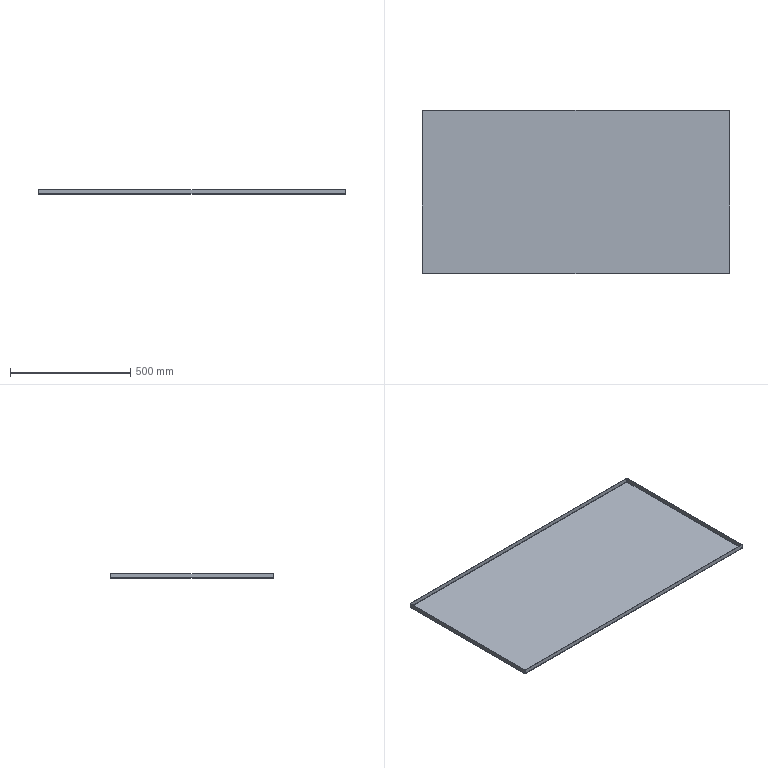Part | STEP file | Part 10 | 1 solid | 38 faces | box 1280 x 680 x 20 mm | volume 1876066 mm3 | plane 22 | spline 8 | cylinder 8 | commonest cylinder face diameters 1 x4 5 x4
STEP:
#1=CARTESIAN_POINT('',(-637.5,-337.5,-2.));
#2=VERTEX_POINT('',#1);
#3=CARTESIAN_POINT('',(-637.5,337.5,-2.));
#4=VERTEX_POINT('',#3);
#5=CARTESIAN_POINT('',(-637.5,-337.5,-2.));
#6=DIRECTION('',(0.,1.,0.));
#7=VECTOR('',#6,1000.);
#8=LINE('',#5,#7);
#9=EDGE_CURVE('',#2,#4,#8,.T.);
#10=ORIENTED_EDGE('',*,*,#9,.T.);
#11=CARTESIAN_POINT('',(637.5,337.5,-2.));
#12=VERTEX_POINT('',#11);
#13=CARTESIAN_POINT('',(-637.5,337.5,-2.));
#14=DIRECTION('',(1.,0.,0.));
#15=VECTOR('',#14,1000.);
#16=LINE('',#13,#15);
#17=EDGE_CURVE('',#4,#12,#16,.T.);
#18=ORIENTED_EDGE('',*,*,#17,.T.);
#19=CARTESIAN_POINT('',(637.5,-337.5,-2.));
#20=VERTEX_POINT('',#19);
#21=CARTESIAN_POINT('',(637.5,337.5,-2.));
#22=DIRECTION('',(0.,-1.,0.));
#23=VECTOR('',#22,1000.);
#24=LINE('',#21,#23);
#25=EDGE_CURVE('',#12,#20,#24,.T.);
#26=ORIENTED_EDGE('',*,*,#25,.T.);
#27=CARTESIAN_POINT('',(637.5,-337.5,-2.));
#28=DIRECTION('',(-1.,0.,0.));
#29=VECTOR('',#28,1000.);
#30=LINE('',#27,#29);
#31=EDGE_CURVE('',#20,#2,#30,.T.);
#32=ORIENTED_EDGE('',*,*,#31,.T.);
#33=EDGE_LOOP('',(#10,#18,#26,#32));
#34=FACE_OUTER_BOUND('',#33,.T.);
#35=CARTESIAN_POINT('',(0.,0.,-2.));
#36=DIRECTION('',(0.,0.,1.));
#37=DIRECTION('',(1.,0.,0.));
#38=AXIS2_PLACEMENT_3D('',#35,#36,#37);
#39=PLANE('',#38);
#40=ADVANCED_FACE('',(#34),#39,.F.);
#41=CARTESIAN_POINT('',(-637.5,337.5,0.));
#42=VERTEX_POINT('',#41);
#43=CARTESIAN_POINT('',(637.5,337.5,0.));
#44=VERTEX_POINT('',#43);
#45=CARTESIAN_POINT('',(-637.5,337.5,0.));
#46=DIRECTION('',(1.,0.,0.));
#47=VECTOR('',#46,1000.);
#48=LINE('',#45,#47);
#49=EDGE_CURVE('',#42,#44,#48,.T.);
#50=ORIENTED_EDGE('',*,*,#49,.F.);
#51=CARTESIAN_POINT('',(-637.5,-337.5,0.));
#52=VERTEX_POINT('',#51);
#53=CARTESIAN_POINT('',(-637.5,-337.5,0.));
#54=DIRECTION('',(0.,1.,0.));
#55=VECTOR('',#54,1000.);
#56=LINE('',#53,#55);
#57=EDGE_CURVE('',#52,#42,#56,.T.);
#58=ORIENTED_EDGE('',*,*,#57,.F.);
#59=CARTESIAN_POINT('',(637.5,-337.5,0.));
#60=VERTEX_POINT('',#59);
#61=CARTESIAN_POINT('',(637.5,-337.5,0.));
#62=DIRECTION('',(-1.,0.,0.));
#63=VECTOR('',#62,1000.);
#64=LINE('',#61,#63);
#65=EDGE_CURVE('',#60,#52,#64,.T.);
#66=ORIENTED_EDGE('',*,*,#65,.F.);
#67=CARTESIAN_POINT('',(637.5,337.5,0.));
#68=DIRECTION('',(0.,-1.,0.));
#69=VECTOR('',#68,1000.);
#70=LINE('',#67,#69);
#71=EDGE_CURVE('',#44,#60,#70,.T.);
#72=ORIENTED_EDGE('',*,*,#71,.F.);
#73=EDGE_LOOP('',(#50,#58,#66,#72));
#74=FACE_OUTER_BOUND('',#73,.T.);
#75=CARTESIAN_POINT('',(0.,0.,0.));
#76=DIRECTION('',(0.,0.,1.));
#77=DIRECTION('',(1.,0.,0.));
#78=AXIS2_PLACEMENT_3D('',#75,#76,#77);
#79=PLANE('',#78);
#80=ADVANCED_FACE('',(#74),#79,.T.);
#81=CARTESIAN_POINT('',(637.293,340.,0.5));
#82=VERTEX_POINT('',#81);
#83=CARTESIAN_POINT('',(637.293,338.,0.5));
#84=VERTEX_POINT('',#83);
#85=CARTESIAN_POINT('',(637.293,338.,0.5));
#86=DIRECTION('',(0.,-1.,0.));
#87=VECTOR('',#86,1000.);
#88=LINE('',#85,#87);
#89=EDGE_CURVE('',#82,#84,#88,.T.);
#90=ORIENTED_EDGE('',*,*,#89,.T.);
#91=CARTESIAN_POINT('',(637.5,337.5,0.));
#92=CARTESIAN_POINT('',(637.465,337.631,0.));
#93=CARTESIAN_POINT('',(637.431,337.761,0.05389));
#94=CARTESIAN_POINT('',(637.362,337.946,0.239));
#95=CARTESIAN_POINT('',(637.327,338.,0.3691));
#96=CARTESIAN_POINT('',(637.293,338.,0.5));
#97=B_SPLINE_CURVE_WITH_KNOTS('',3,(#91,#92,#93,#94,#95,#96),.UNSPECIFIED.,.F.,.F.,(4,2,4),(0.,0.5,1.),.UNSPECIFIED.);
#98=EDGE_CURVE('',#44,#84,#97,.T.);
#99=ORIENTED_EDGE('',*,*,#98,.F.);
#100=CARTESIAN_POINT('',(637.5,337.5,0.));
#101=DIRECTION('',(0.,0.,-1.));
#102=VECTOR('',#101,1000.);
#103=LINE('',#100,#102);
#104=EDGE_CURVE('',#44,#12,#103,.T.);
#105=ORIENTED_EDGE('',*,*,#104,.T.);
#106=CARTESIAN_POINT('',(637.5,337.5,-2.));
#107=CARTESIAN_POINT('',(637.483,337.827,-2.));
#108=CARTESIAN_POINT('',(637.465,338.154,-1.935));
#109=CARTESIAN_POINT('',(637.431,338.759,-1.684));
#110=CARTESIAN_POINT('',(637.414,339.036,-1.499));
#111=CARTESIAN_POINT('',(637.379,339.499,-1.036));
#112=CARTESIAN_POINT('',(637.362,339.684,-0.759));
#113=CARTESIAN_POINT('',(637.327,339.935,-0.1544));
#114=CARTESIAN_POINT('',(637.31,340.,0.1728));
#115=CARTESIAN_POINT('',(637.293,340.,0.5));
#116=B_SPLINE_CURVE_WITH_KNOTS('',3,(#106,#107,#108,#109,#110,#111,#112,#113,#114,#115),.UNSPECIFIED.,.F.,.F.,(4,2,2,2,4),(0.,0.25,0.5,0.75,1.),.UNSPECIFIED.);
#117=EDGE_CURVE('',#12,#82,#116,.T.);
#118=ORIENTED_EDGE('',*,*,#117,.T.);
#119=EDGE_LOOP('',(#90,#99,#105,#118));
#120=FACE_OUTER_BOUND('',#119,.T.);
#121=CARTESIAN_POINT('',(637.5,337.5,-2.02));
#122=CARTESIAN_POINT('',(637.483,337.83,-2.02));
#123=CARTESIAN_POINT('',(637.465,338.16,-1.954));
#124=CARTESIAN_POINT('',(637.431,338.769,-1.702));
#125=CARTESIAN_POINT('',(637.414,339.049,-1.515));
#126=CARTESIAN_POINT('',(637.379,339.515,-1.049));
#127=CARTESIAN_POINT('',(637.362,339.702,-0.7691));
#128=CARTESIAN_POINT('',(637.327,339.954,-0.1596));
#129=CARTESIAN_POINT('',(637.31,340.02,0.1701));
#130=CARTESIAN_POINT('',(637.293,340.02,0.5));
#131=CARTESIAN_POINT('',(637.5,337.5,-2.));
#132=CARTESIAN_POINT('',(637.483,337.827,-2.));
#133=CARTESIAN_POINT('',(637.465,338.154,-1.935));
#134=CARTESIAN_POINT('',(637.431,338.759,-1.684));
#135=CARTESIAN_POINT('',(637.414,339.036,-1.499));
#136=CARTESIAN_POINT('',(637.379,339.499,-1.036));
#137=CARTESIAN_POINT('',(637.362,339.684,-0.759));
#138=CARTESIAN_POINT('',(637.327,339.935,-0.1544));
#139=CARTESIAN_POINT('',(637.31,340.,0.1727));
#140=CARTESIAN_POINT('',(637.293,340.,0.5));
#141=CARTESIAN_POINT('',(637.5,337.5,0.));
#142=CARTESIAN_POINT('',(637.483,337.565,0.));
#143=CARTESIAN_POINT('',(637.465,337.631,0.01301));
#144=CARTESIAN_POINT('',(637.431,337.752,0.06311));
#145=CARTESIAN_POINT('',(637.414,337.807,0.1002));
#146=CARTESIAN_POINT('',(637.379,337.9,0.1927));
#147=CARTESIAN_POINT('',(637.362,337.937,0.2482));
#148=CARTESIAN_POINT('',(637.327,337.987,0.3691));
#149=CARTESIAN_POINT('',(637.31,338.,0.4345));
#150=CARTESIAN_POINT('',(637.293,338.,0.5));
#151=CARTESIAN_POINT('',(637.5,337.5,0.0202));
#152=CARTESIAN_POINT('',(637.483,337.563,0.0202));
#153=CARTESIAN_POINT('',(637.465,337.626,0.03269));
#154=CARTESIAN_POINT('',(637.431,337.742,0.08076));
#155=CARTESIAN_POINT('',(637.414,337.795,0.1163));
#156=CARTESIAN_POINT('',(637.379,337.884,0.2051));
#157=CARTESIAN_POINT('',(637.362,337.919,0.2584));
#158=CARTESIAN_POINT('',(637.327,337.967,0.3744));
#159=CARTESIAN_POINT('',(637.31,337.98,0.4372));
#160=CARTESIAN_POINT('',(637.293,337.98,0.5));
#161=B_SPLINE_SURFACE_WITH_KNOTS('',1,3,((#121,#122,#123,#124,#125,#126,#127,#128,#129,#130),(#131,#132,#133,#134,#135,#136,#137,#138,#139,#140),(#141,#142,#143,#144,#145,#146,#147,#148,#149,#150),(#151,#152,#153,#154,#155,#156,#157,#158,#159,#160)),.UNSPECIFIED.,.F.,.F.,.F.,(2,1,1,2),(4,2,2,2,4),(-0.01,0.,1.,1.01),(0.,0.25,0.5,0.75,1.),.UNSPECIFIED.);
#162=ADVANCED_FACE('',(#120),#161,.F.);
#163=CARTESIAN_POINT('',(-637.293,338.,0.5));
#164=VERTEX_POINT('',#163);
#165=CARTESIAN_POINT('',(-637.293,338.,0.5));
#166=CARTESIAN_POINT('',(-637.327,338.,0.3691));
#167=CARTESIAN_POINT('',(-637.362,337.946,0.239));
#168=CARTESIAN_POINT('',(-637.431,337.761,0.05389));
#169=CARTESIAN_POINT('',(-637.465,337.631,0.));
#170=CARTESIAN_POINT('',(-637.5,337.5,0.));
#171=B_SPLINE_CURVE_WITH_KNOTS('',3,(#165,#166,#167,#168,#169,#170),.UNSPECIFIED.,.F.,.F.,(4,2,4),(0.,0.5,1.),.UNSPECIFIED.);
#172=EDGE_CURVE('',#164,#42,#171,.T.);
#173=ORIENTED_EDGE('',*,*,#172,.F.);
#174=CARTESIAN_POINT('',(-637.293,340.,0.5));
#175=VERTEX_POINT('',#174);
#176=CARTESIAN_POINT('',(-637.293,338.,0.5));
#177=DIRECTION('',(0.,-1.,0.));
#178=VECTOR('',#177,1000.);
#179=LINE('',#176,#178);
#180=EDGE_CURVE('',#175,#164,#179,.T.);
#181=ORIENTED_EDGE('',*,*,#180,.F.);
#182=CARTESIAN_POINT('',(-637.293,340.,0.5));
#183=CARTESIAN_POINT('',(-637.31,340.,0.1728));
#184=CARTESIAN_POINT('',(-637.327,339.935,-0.1544));
#185=CARTESIAN_POINT('',(-637.362,339.684,-0.759));
#186=CARTESIAN_POINT('',(-637.379,339.499,-1.036));
#187=CARTESIAN_POINT('',(-637.414,339.036,-1.499));
#188=CARTESIAN_POINT('',(-637.431,338.759,-1.684));
#189=CARTESIAN_POINT('',(-637.465,338.154,-1.935));
#190=CARTESIAN_POINT('',(-637.483,337.827,-2.));
#191=CARTESIAN_POINT('',(-637.5,337.5,-2.));
#192=B_SPLINE_CURVE_WITH_KNOTS('',3,(#182,#183,#184,#185,#186,#187,#188,#189,#190,#191),.UNSPECIFIED.,.F.,.F.,(4,2,2,2,4),(0.,0.25,0.5,0.75,1.),.UNSPECIFIED.);
#193=EDGE_CURVE('',#175,#4,#192,.T.);
#194=ORIENTED_EDGE('',*,*,#193,.T.);
#195=CARTESIAN_POINT('',(-637.5,337.5,0.));
#196=DIRECTION('',(0.,0.,-1.));
#197=VECTOR('',#196,1000.);
#198=LINE('',#195,#197);
#199=EDGE_CURVE('',#42,#4,#198,.T.);
#200=ORIENTED_EDGE('',*,*,#199,.F.);
#201=EDGE_LOOP('',(#173,#181,#194,#200));
#202=FACE_OUTER_BOUND('',#201,.T.);
#203=CARTESIAN_POINT('',(-637.293,340.02,0.5));
#204=CARTESIAN_POINT('',(-637.31,340.02,0.1701));
#205=CARTESIAN_POINT('',(-637.327,339.954,-0.1596));
#206=CARTESIAN_POINT('',(-637.362,339.702,-0.7691));
#207=CARTESIAN_POINT('',(-637.379,339.515,-1.049));
#208=CARTESIAN_POINT('',(-637.414,339.049,-1.515));
#209=CARTESIAN_POINT('',(-637.431,338.769,-1.702));
#210=CARTESIAN_POINT('',(-637.465,338.16,-1.954));
#211=CARTESIAN_POINT('',(-637.483,337.83,-2.02));
#212=CARTESIAN_POINT('',(-637.5,337.5,-2.02));
#213=CARTESIAN_POINT('',(-637.293,340.,0.5));
#214=CARTESIAN_POINT('',(-637.31,340.,0.1727));
#215=CARTESIAN_POINT('',(-637.327,339.935,-0.1544));
#216=CARTESIAN_POINT('',(-637.362,339.684,-0.759));
#217=CARTESIAN_POINT('',(-637.379,339.499,-1.036));
#218=CARTESIAN_POINT('',(-637.414,339.036,-1.499));
#219=CARTESIAN_POINT('',(-637.431,338.759,-1.684));
#220=CARTESIAN_POINT('',(-637.465,338.154,-1.935));
#221=CARTESIAN_POINT('',(-637.483,337.827,-2.));
#222=CARTESIAN_POINT('',(-637.5,337.5,-2.));
#223=CARTESIAN_POINT('',(-637.293,338.,0.5));
#224=CARTESIAN_POINT('',(-637.31,338.,0.4345));
#225=CARTESIAN_POINT('',(-637.327,337.987,0.3691));
#226=CARTESIAN_POINT('',(-637.362,337.937,0.2482));
#227=CARTESIAN_POINT('',(-637.379,337.9,0.1927));
#228=CARTESIAN_POINT('',(-637.414,337.807,0.1002));
#229=CARTESIAN_POINT('',(-637.431,337.752,0.06311));
#230=CARTESIAN_POINT('',(-637.465,337.631,0.01301));
#231=CARTESIAN_POINT('',(-637.483,337.565,0.));
#232=CARTESIAN_POINT('',(-637.5,337.5,0.));
#233=CARTESIAN_POINT('',(-637.293,337.98,0.5));
#234=CARTESIAN_POINT('',(-637.31,337.98,0.4372));
#235=CARTESIAN_POINT('',(-637.327,337.967,0.3744));
#236=CARTESIAN_POINT('',(-637.362,337.919,0.2584));
#237=CARTESIAN_POINT('',(-637.379,337.884,0.2051));
#238=CARTESIAN_POINT('',(-637.414,337.795,0.1163));
#239=CARTESIAN_POINT('',(-637.431,337.742,0.08076));
#240=CARTESIAN_POINT('',(-637.465,337.626,0.03269));
#241=CARTESIAN_POINT('',(-637.483,337.563,0.0202));
#242=CARTESIAN_POINT('',(-637.5,337.5,0.0202));
#243=B_SPLINE_SURFACE_WITH_KNOTS('',1,3,((#203,#204,#205,#206,#207,#208,#209,#210,#211,#212),(#213,#214,#215,#216,#217,#218,#219,#220,#221,#222),(#223,#224,#225,#226,#227,#228,#229,#230,#231,#232),(#233,#234,#235,#236,#237,#238,#239,#240,#241,#242)),.UNSPECIFIED.,.F.,.F.,.F.,(2,1,1,2),(4,2,2,2,4),(-0.01,0.,1.,1.01),(0.,0.25,0.5,0.75,1.),.UNSPECIFIED.);
#244=ADVANCED_FACE('',(#202),#243,.F.);
#245=ORIENTED_EDGE('',*,*,#17,.F.);
#246=ORIENTED_EDGE('',*,*,#193,.F.);
#247=CARTESIAN_POINT('',(0.,340.,0.5));
#248=DIRECTION('',(-1.,0.,0.));
#249=VECTOR('',#248,1000.);
#250=LINE('',#247,#249);
#251=EDGE_CURVE('',#82,#175,#250,.T.);
#252=ORIENTED_EDGE('',*,*,#251,.F.);
#253=ORIENTED_EDGE('',*,*,#117,.F.);
#254=EDGE_LOOP('',(#245,#246,#252,#253));
#255=FACE_OUTER_BOUND('',#254,.T.);
#256=CARTESIAN_POINT('',(-637.5,337.5,0.5));
#257=DIRECTION('',(-1.,0.,0.));
#258=DIRECTION('',(0.,1.,0.));
#259=AXIS2_PLACEMENT_3D('',#256,#257,#258);
#260=CYLINDRICAL_SURFACE('',#259,2.5);
#261=ADVANCED_FACE('',(#255),#260,.T.);
#262=ORIENTED_EDGE('',*,*,#49,.T.);
#263=ORIENTED_EDGE('',*,*,#98,.T.);
#264=CARTESIAN_POINT('',(640.,338.,0.5));
#265=DIRECTION('',(-1.,0.,0.));
#266=VECTOR('',#265,1000.);
#267=LINE('',#264,#266);
#268=EDGE_CURVE('',#84,#164,#267,.T.);
#269=ORIENTED_EDGE('',*,*,#268,.T.);
#270=ORIENTED_EDGE('',*,*,#172,.T.);
#271=EDGE_LOOP('',(#262,#263,#269,#270));
#272=FACE_OUTER_BOUND('',#271,.T.);
#273=CARTESIAN_POINT('',(-637.5,337.5,0.5));
#274=DIRECTION('',(-1.,0.,0.));
#275=DIRECTION('',(0.,1.,0.));
#276=AXIS2_PLACEMENT_3D('',#273,#274,#275);
#277=CYLINDRICAL_SURFACE('',#276,0.5);
#278=ADVANCED_FACE('',(#272),#277,.F.);
#279=CARTESIAN_POINT('',(637.293,338.,18.));
#280=VERTEX_POINT('',#279);
#281=CARTESIAN_POINT('',(637.293,340.,18.));
#282=VERTEX_POINT('',#281);
#283=CARTESIAN_POINT('',(637.293,340.,18.));
#284=DIRECTION('',(0.,1.,0.));
#285=VECTOR('',#284,1000.);
#286=LINE('',#283,#285);
#287=EDGE_CURVE('',#280,#282,#286,.T.);
#288=ORIENTED_EDGE('',*,*,#287,.F.);
#289=CARTESIAN_POINT('',(637.293,338.,0.));
#290=DIRECTION('',(0.,0.,1.));
#291=VECTOR('',#290,1000.);
#292=LINE('',#289,#291);
#293=EDGE_CURVE('',#84,#280,#292,.T.);
#294=ORIENTED_EDGE('',*,*,#293,.F.);
#295=ORIENTED_EDGE('',*,*,#89,.F.);
#296=CARTESIAN_POINT('',(637.293,340.,0.));
#297=DIRECTION('',(0.,0.,-1.));
#298=VECTOR('',#297,1000.);
#299=LINE('',#296,#298);
#300=EDGE_CURVE('',#282,#82,#299,.T.);
#301=ORIENTED_EDGE('',*,*,#300,.F.);
#302=EDGE_LOOP('',(#288,#294,#295,#301));
#303=FACE_OUTER_BOUND('',#302,.T.);
#304=CARTESIAN_POINT('',(637.293,338.,0.));
#305=DIRECTION('',(1.,0.,0.));
#306=DIRECTION('',(0.,0.,-1.));
#307=AXIS2_PLACEMENT_3D('',#304,#305,#306);
#308=PLANE('',#307);
#309=ADVANCED_FACE('',(#303),#308,.T.);
#310=CARTESIAN_POINT('',(-637.293,340.,18.));
#311=VERTEX_POINT('',#310);
#312=CARTESIAN_POINT('',(-637.293,340.,0.));
#313=DIRECTION('',(0.,0.,-1.));
#314=VECTOR('',#313,1000.);
#315=LINE('',#312,#314);
#316=EDGE_CURVE('',#311,#175,#315,.T.);
#317=ORIENTED_EDGE('',*,*,#316,.F.);
#318=CARTESIAN_POINT('',(-640.,340.,18.));
#319=DIRECTION('',(-1.,0.,0.));
#320=VECTOR('',#319,1000.);
#321=LINE('',#318,#320);
#322=EDGE_CURVE('',#282,#311,#321,.T.);
#323=ORIENTED_EDGE('',*,*,#322,.F.);
#324=ORIENTED_EDGE('',*,*,#300,.T.);
#325=ORIENTED_EDGE('',*,*,#251,.T.);
#326=EDGE_LOOP('',(#317,#323,#324,#325));
#327=FACE_OUTER_BOUND('',#326,.T.);
#328=CARTESIAN_POINT('',(0.,340.,0.));
#329=DIRECTION('',(0.,1.,0.));
#330=DIRECTION('',(0.,0.,1.));
#331=AXIS2_PLACEMENT_3D('',#328,#329,#330);
#332=PLANE('',#331);
#333=ADVANCED_FACE('',(#327),#332,.T.);
#334=CARTESIAN_POINT('',(-637.293,338.,18.));
#335=VERTEX_POINT('',#334);
#336=CARTESIAN_POINT('',(0.,338.,18.));
#337=DIRECTION('',(-1.,0.,0.));
#338=VECTOR('',#337,1000.);
#339=LINE('',#336,#338);
#340=EDGE_CURVE('',#280,#335,#339,.T.);
#341=ORIENTED_EDGE('',*,*,#340,.T.);
#342=CARTESIAN_POINT('',(-637.293,338.,0.));
#343=DIRECTION('',(0.,0.,1.));
#344=VECTOR('',#343,1000.);
#345=LINE('',#342,#344);
#346=EDGE_CURVE('',#164,#335,#345,.T.);
#347=ORIENTED_EDGE('',*,*,#346,.F.);
#348=ORIENTED_EDGE('',*,*,#268,.F.);
#349=ORIENTED_EDGE('',*,*,#293,.T.);
#350=EDGE_LOOP('',(#341,#347,#348,#349));
#351=FACE_OUTER_BOUND('',#350,.T.);
#352=CARTESIAN_POINT('',(0.,338.,0.));
#353=DIRECTION('',(0.,1.,0.));
#354=DIRECTION('',(0.,0.,1.));
#355=AXIS2_PLACEMENT_3D('',#352,#353,#354);
#356=PLANE('',#355);
#357=ADVANCED_FACE('',(#351),#356,.F.);
#358=CARTESIAN_POINT('',(-637.293,338.,18.));
#359=DIRECTION('',(0.,1.,0.));
#360=VECTOR('',#359,1000.);
#361=LINE('',#358,#360);
#362=EDGE_CURVE('',#335,#311,#361,.T.);
#363=ORIENTED_EDGE('',*,*,#362,.F.);
#364=ORIENTED_EDGE('',*,*,#340,.F.);
#365=ORIENTED_EDGE('',*,*,#287,.T.);
#366=ORIENTED_EDGE('',*,*,#322,.T.);
#367=EDGE_LOOP('',(#363,#364,#365,#366));
#368=FACE_OUTER_BOUND('',#367,.T.);
#369=CARTESIAN_POINT('',(-640.,340.,18.));
#370=DIRECTION('',(0.,0.,1.));
#371=DIRECTION('',(0.,-1.,0.));
#372=AXIS2_PLACEMENT_3D('',#369,#370,#371);
#373=PLANE('',#372);
#374=ADVANCED_FACE('',(#368),#373,.T.);
#375=ORIENTED_EDGE('',*,*,#346,.T.);
#376=ORIENTED_EDGE('',*,*,#362,.T.);
#377=ORIENTED_EDGE('',*,*,#316,.T.);
#378=ORIENTED_EDGE('',*,*,#180,.T.);
#379=EDGE_LOOP('',(#375,#376,#377,#378));
#380=FACE_OUTER_BOUND('',#379,.T.);
#381=CARTESIAN_POINT('',(-637.293,338.,0.));
#382=DIRECTION('',(1.,0.,0.));
#383=DIRECTION('',(0.,0.,-1.));
#384=AXIS2_PLACEMENT_3D('',#381,#382,#383);
#385=PLANE('',#384);
#386=ADVANCED_FACE('',(#380),#385,.F.);
#387=CARTESIAN_POINT('',(640.,-337.293,0.5));
#388=VERTEX_POINT('',#387);
#389=CARTESIAN_POINT('',(638.,-337.293,0.5));
#390=VERTEX_POINT('',#389);
#391=CARTESIAN_POINT('',(638.,-337.293,0.5));
#392=DIRECTION('',(-1.,0.,0.));
#393=VECTOR('',#392,1000.);
#394=LINE('',#391,#393);
#395=EDGE_CURVE('',#388,#390,#394,.T.);
#396=ORIENTED_EDGE('',*,*,#395,.T.);
#397=CARTESIAN_POINT('',(637.5,-337.5,0.));
#398=CARTESIAN_POINT('',(637.631,-337.465,0.));
#399=CARTESIAN_POINT('',(637.761,-337.431,0.05389));
#400=CARTESIAN_POINT('',(637.946,-337.362,0.239));
#401=CARTESIAN_POINT('',(638.,-337.327,0.3691));
#402=CARTESIAN_POINT('',(638.,-337.293,0.5));
#403=B_SPLINE_CURVE_WITH_KNOTS('',3,(#397,#398,#399,#400,#401,#402),.UNSPECIFIED.,.F.,.F.,(4,2,4),(0.,0.5,1.),.UNSPECIFIED.);
#404=EDGE_CURVE('',#60,#390,#403,.T.);
#405=ORIENTED_EDGE('',*,*,#404,.F.);
#406=CARTESIAN_POINT('',(637.5,-337.5,0.));
#407=DIRECTION('',(0.,0.,-1.));
#408=VECTOR('',#407,1000.);
#409=LINE('',#406,#408);
#410=EDGE_CURVE('',#60,#20,#409,.T.);
#411=ORIENTED_EDGE('',*,*,#410,.T.);
#412=CARTESIAN_POINT('',(637.5,-337.5,-2.));
#413=CARTESIAN_POINT('',(637.827,-337.483,-2.));
#414=CARTESIAN_POINT('',(638.154,-337.465,-1.935));
#415=CARTESIAN_POINT('',(638.759,-337.431,-1.684));
#416=CARTESIAN_POINT('',(639.036,-337.414,-1.499));
#417=CARTESIAN_POINT('',(639.499,-337.379,-1.036));
#418=CARTESIAN_POINT('',(639.684,-337.362,-0.759));
#419=CARTESIAN_POINT('',(639.935,-337.327,-0.1544));
#420=CARTESIAN_POINT('',(640.,-337.31,0.1728));
#421=CARTESIAN_POINT('',(640.,-337.293,0.5));
#422=B_SPLINE_CURVE_WITH_KNOTS('',3,(#412,#413,#414,#415,#416,#417,#418,#419,#420,#421),.UNSPECIFIED.,.F.,.F.,(4,2,2,2,4),(0.,0.25,0.5,0.75,1.),.UNSPECIFIED.);
#423=EDGE_CURVE('',#20,#388,#422,.T.);
#424=ORIENTED_EDGE('',*,*,#423,.T.);
#425=EDGE_LOOP('',(#396,#405,#411,#424));
#426=FACE_OUTER_BOUND('',#425,.T.);
#427=CARTESIAN_POINT('',(637.5,-337.5,-2.02));
#428=CARTESIAN_POINT('',(637.83,-337.483,-2.02));
#429=CARTESIAN_POINT('',(638.16,-337.465,-1.954));
#430=CARTESIAN_POINT('',(638.769,-337.431,-1.702));
#431=CARTESIAN_POINT('',(639.049,-337.414,-1.515));
#432=CARTESIAN_POINT('',(639.515,-337.379,-1.049));
#433=CARTESIAN_POINT('',(639.702,-337.362,-0.7691));
#434=CARTESIAN_POINT('',(639.954,-337.327,-0.1596));
#435=CARTESIAN_POINT('',(640.02,-337.31,0.1701));
#436=CARTESIAN_POINT('',(640.02,-337.293,0.5));
#437=CARTESIAN_POINT('',(637.5,-337.5,-2.));
#438=CARTESIAN_POINT('',(637.827,-337.483,-2.));
#439=CARTESIAN_POINT('',(638.154,-337.465,-1.935));
#440=CARTESIAN_POINT('',(638.759,-337.431,-1.684));
#441=CARTESIAN_POINT('',(639.036,-337.414,-1.499));
#442=CARTESIAN_POINT('',(639.499,-337.379,-1.036));
#443=CARTESIAN_POINT('',(639.684,-337.362,-0.759));
#444=CARTESIAN_POINT('',(639.935,-337.327,-0.1544));
#445=CARTESIAN_POINT('',(640.,-337.31,0.1727));
#446=CARTESIAN_POINT('',(640.,-337.293,0.5));
#447=CARTESIAN_POINT('',(637.5,-337.5,0.));
#448=CARTESIAN_POINT('',(637.565,-337.483,0.));
#449=CARTESIAN_POINT('',(637.631,-337.465,0.01301));
#450=CARTESIAN_POINT('',(637.752,-337.431,0.06311));
#451=CARTESIAN_POINT('',(637.807,-337.414,0.1002));
#452=CARTESIAN_POINT('',(637.9,-337.379,0.1927));
#453=CARTESIAN_POINT('',(637.937,-337.362,0.2482));
#454=CARTESIAN_POINT('',(637.987,-337.327,0.3691));
#455=CARTESIAN_POINT('',(638.,-337.31,0.4345));
#456=CARTESIAN_POINT('',(638.,-337.293,0.5));
#457=CARTESIAN_POINT('',(637.5,-337.5,0.0202));
#458=CARTESIAN_POINT('',(637.563,-337.483,0.0202));
#459=CARTESIAN_POINT('',(637.626,-337.465,0.03269));
#460=CARTESIAN_POINT('',(637.742,-337.431,0.08076));
#461=CARTESIAN_POINT('',(637.795,-337.414,0.1163));
#462=CARTESIAN_POINT('',(637.884,-337.379,0.2051));
#463=CARTESIAN_POINT('',(637.919,-337.362,0.2584));
#464=CARTESIAN_POINT('',(637.967,-337.327,0.3744));
#465=CARTESIAN_POINT('',(637.98,-337.31,0.4372));
#466=CARTESIAN_POINT('',(637.98,-337.293,0.5));
#467=B_SPLINE_SURFACE_WITH_KNOTS('',1,3,((#427,#428,#429,#430,#431,#432,#433,#434,#435,#436),(#437,#438,#439,#440,#441,#442,#443,#444,#445,#446),(#447,#448,#449,#450,#451,#452,#453,#454,#455,#456),(#457,#458,#459,#460,#461,#462,#463,#464,#465,#466)),.UNSPECIFIED.,.F.,.F.,.F.,(2,1,1,2),(4,2,2,2,4),(-0.01,0.,1.,1.01),(0.,0.25,0.5,0.75,1.),.UNSPECIFIED.);
#468=ADVANCED_FACE('',(#426),#467,.F.);
#469=CARTESIAN_POINT('',(638.,337.293,0.5));
#470=VERTEX_POINT('',#469);
#471=CARTESIAN_POINT('',(638.,337.293,0.5));
#472=CARTESIAN_POINT('',(638.,337.327,0.3691));
#473=CARTESIAN_POINT('',(637.946,337.362,0.239));
#474=CARTESIAN_POINT('',(637.761,337.431,0.05389));
#475=CARTESIAN_POINT('',(637.631,337.465,0.));
#476=CARTESIAN_POINT('',(637.5,337.5,0.));
#477=B_SPLINE_CURVE_WITH_KNOTS('',3,(#471,#472,#473,#474,#475,#476),.UNSPECIFIED.,.F.,.F.,(4,2,4),(0.,0.5,1.),.UNSPECIFIED.);
#478=EDGE_CURVE('',#470,#44,#477,.T.);
#479=ORIENTED_EDGE('',*,*,#478,.F.);
#480=CARTESIAN_POINT('',(640.,337.293,0.5));
#481=VERTEX_POINT('',#480);
#482=CARTESIAN_POINT('',(638.,337.293,0.5));
#483=DIRECTION('',(-1.,0.,0.));
#484=VECTOR('',#483,1000.);
#485=LINE('',#482,#484);
#486=EDGE_CURVE('',#481,#470,#485,.T.);
#487=ORIENTED_EDGE('',*,*,#486,.F.);
#488=CARTESIAN_POINT('',(640.,337.293,0.5));
#489=CARTESIAN_POINT('',(640.,337.31,0.1728));
#490=CARTESIAN_POINT('',(639.935,337.327,-0.1544));
#491=CARTESIAN_POINT('',(639.684,337.362,-0.759));
#492=CARTESIAN_POINT('',(639.499,337.379,-1.036));
#493=CARTESIAN_POINT('',(639.036,337.414,-1.499));
#494=CARTESIAN_POINT('',(638.759,337.431,-1.684));
#495=CARTESIAN_POINT('',(638.154,337.465,-1.935));
#496=CARTESIAN_POINT('',(637.827,337.483,-2.));
#497=CARTESIAN_POINT('',(637.5,337.5,-2.));
#498=B_SPLINE_CURVE_WITH_KNOTS('',3,(#488,#489,#490,#491,#492,#493,#494,#495,#496,#497),.UNSPECIFIED.,.F.,.F.,(4,2,2,2,4),(0.,0.25,0.5,0.75,1.),.UNSPECIFIED.);
#499=EDGE_CURVE('',#481,#12,#498,.T.);
#500=ORIENTED_EDGE('',*,*,#499,.T.);
#501=ORIENTED_EDGE('',*,*,#104,.F.);
#502=EDGE_LOOP('',(#479,#487,#500,#501));
#503=FACE_OUTER_BOUND('',#502,.T.);
#504=CARTESIAN_POINT('',(640.02,337.293,0.5));
#505=CARTESIAN_POINT('',(640.02,337.31,0.1701));
#506=CARTESIAN_POINT('',(639.954,337.327,-0.1596));
#507=CARTESIAN_POINT('',(639.702,337.362,-0.7691));
#508=CARTESIAN_POINT('',(639.515,337.379,-1.049));
#509=CARTESIAN_POINT('',(639.049,337.414,-1.515));
#510=CARTESIAN_POINT('',(638.769,337.431,-1.702));
#511=CARTESIAN_POINT('',(638.16,337.465,-1.954));
#512=CARTESIAN_POINT('',(637.83,337.483,-2.02));
#513=CARTESIAN_POINT('',(637.5,337.5,-2.02));
#514=CARTESIAN_POINT('',(640.,337.293,0.5));
#515=CARTESIAN_POINT('',(640.,337.31,0.1727));
#516=CARTESIAN_POINT('',(639.935,337.327,-0.1544));
#517=CARTESIAN_POINT('',(639.684,337.362,-0.759));
#518=CARTESIAN_POINT('',(639.499,337.379,-1.036));
#519=CARTESIAN_POINT('',(639.036,337.414,-1.499));
#520=CARTESIAN_POINT('',(638.759,337.431,-1.684));
#521=CARTESIAN_POINT('',(638.154,337.465,-1.935));
#522=CARTESIAN_POINT('',(637.827,337.483,-2.));
#523=CARTESIAN_POINT('',(637.5,337.5,-2.));
#524=CARTESIAN_POINT('',(638.,337.293,0.5));
#525=CARTESIAN_POINT('',(638.,337.31,0.4345));
#526=CARTESIAN_POINT('',(637.987,337.327,0.3691));
#527=CARTESIAN_POINT('',(637.937,337.362,0.2482));
#528=CARTESIAN_POINT('',(637.9,337.379,0.1927));
#529=CARTESIAN_POINT('',(637.807,337.414,0.1002));
#530=CARTESIAN_POINT('',(637.752,337.431,0.06311));
#531=CARTESIAN_POINT('',(637.631,337.465,0.01301));
#532=CARTESIAN_POINT('',(637.565,337.483,0.));
#533=CARTESIAN_POINT('',(637.5,337.5,0.));
#534=CARTESIAN_POINT('',(637.98,337.293,0.5));
#535=CARTESIAN_POINT('',(637.98,337.31,0.4372));
#536=CARTESIAN_POINT('',(637.967,337.327,0.3744));
#537=CARTESIAN_POINT('',(637.919,337.362,0.2584));
#538=CARTESIAN_POINT('',(637.884,337.379,0.2051));
#539=CARTESIAN_POINT('',(637.795,337.414,0.1163));
#540=CARTESIAN_POINT('',(637.742,337.431,0.08076));
#541=CARTESIAN_POINT('',(637.626,337.465,0.03269));
#542=CARTESIAN_POINT('',(637.563,337.483,0.0202));
#543=CARTESIAN_POINT('',(637.5,337.5,0.0202));
#544=B_SPLINE_SURFACE_WITH_KNOTS('',1,3,((#504,#505,#506,#507,#508,#509,#510,#511,#512,#513),(#514,#515,#516,#517,#518,#519,#520,#521,#522,#523),(#524,#525,#526,#527,#528,#529,#530,#531,#532,#533),(#534,#535,#536,#537,#538,#539,#540,#541,#542,#543)),.UNSPECIFIED.,.F.,.F.,.F.,(2,1,1,2),(4,2,2,2,4),(-0.01,0.,1.,1.01),(0.,0.25,0.5,0.75,1.),.UNSPECIFIED.);
#545=ADVANCED_FACE('',(#503),#544,.F.);
#546=ORIENTED_EDGE('',*,*,#25,.F.);
#547=ORIENTED_EDGE('',*,*,#499,.F.);
#548=CARTESIAN_POINT('',(640.,-340.,0.5));
#549=DIRECTION('',(0.,-1.,0.));
#550=VECTOR('',#549,1000.);
#551=LINE('',#548,#550);
#552=EDGE_CURVE('',#481,#388,#551,.T.);
#553=ORIENTED_EDGE('',*,*,#552,.T.);
#554=ORIENTED_EDGE('',*,*,#423,.F.);
#555=EDGE_LOOP('',(#546,#547,#553,#554));
#556=FACE_OUTER_BOUND('',#555,.T.);
#557=CARTESIAN_POINT('',(637.5,337.5,0.5));
#558=DIRECTION('',(0.,1.,0.));
#559=DIRECTION('',(1.,0.,0.));
#560=AXIS2_PLACEMENT_3D('',#557,#558,#559);
#561=CYLINDRICAL_SURFACE('',#560,2.5);
#562=ADVANCED_FACE('',(#556),#561,.T.);
#563=ORIENTED_EDGE('',*,*,#71,.T.);
#564=ORIENTED_EDGE('',*,*,#404,.T.);
#565=CARTESIAN_POINT('',(638.,-340.,0.5));
#566=DIRECTION('',(0.,1.,0.));
#567=VECTOR('',#566,1000.);
#568=LINE('',#565,#567);
#569=EDGE_CURVE('',#390,#470,#568,.T.);
#570=ORIENTED_EDGE('',*,*,#569,.T.);
#571=ORIENTED_EDGE('',*,*,#478,.T.);
#572=EDGE_LOOP('',(#563,#564,#570,#571));
#573=FACE_OUTER_BOUND('',#572,.T.);
#574=CARTESIAN_POINT('',(637.5,337.5,0.5));
#575=DIRECTION('',(0.,1.,0.));
#576=DIRECTION('',(1.,0.,0.));
#577=AXIS2_PLACEMENT_3D('',#574,#575,#576);
#578=CYLINDRICAL_SURFACE('',#577,0.5);
#579=ADVANCED_FACE('',(#573),#578,.F.);
#580=CARTESIAN_POINT('',(638.,-337.293,18.));
#581=VERTEX_POINT('',#580);
#582=CARTESIAN_POINT('',(640.,-337.293,18.));
#583=VERTEX_POINT('',#582);
#584=CARTESIAN_POINT('',(640.,-337.293,18.));
#585=DIRECTION('',(1.,0.,0.));
#586=VECTOR('',#585,1000.);
#587=LINE('',#584,#586);
#588=EDGE_CURVE('',#581,#583,#587,.T.);
#589=ORIENTED_EDGE('',*,*,#588,.F.);
#590=CARTESIAN_POINT('',(638.,-337.293,0.));
#591=DIRECTION('',(0.,0.,1.));
#592=VECTOR('',#591,1000.);
#593=LINE('',#590,#592);
#594=EDGE_CURVE('',#390,#581,#593,.T.);
#595=ORIENTED_EDGE('',*,*,#594,.F.);
#596=ORIENTED_EDGE('',*,*,#395,.F.);
#597=CARTESIAN_POINT('',(640.,-337.293,0.));
#598=DIRECTION('',(0.,0.,1.));
#599=VECTOR('',#598,1000.);
#600=LINE('',#597,#599);
#601=EDGE_CURVE('',#388,#583,#600,.T.);
#602=ORIENTED_EDGE('',*,*,#601,.T.);
#603=EDGE_LOOP('',(#589,#595,#596,#602));
#604=FACE_OUTER_BOUND('',#603,.T.);
#605=CARTESIAN_POINT('',(638.,-337.293,0.));
#606=DIRECTION('',(0.,-1.,0.));
#607=DIRECTION('',(0.,0.,-1.));
#608=AXIS2_PLACEMENT_3D('',#605,#606,#607);
#609=PLANE('',#608);
#610=ADVANCED_FACE('',(#604),#609,.T.);
#611=ORIENTED_EDGE('',*,*,#552,.F.);
#612=CARTESIAN_POINT('',(640.,337.293,18.));
#613=VERTEX_POINT('',#612);
#614=CARTESIAN_POINT('',(640.,337.293,0.));
#615=DIRECTION('',(0.,0.,1.));
#616=VECTOR('',#615,1000.);
#617=LINE('',#614,#616);
#618=EDGE_CURVE('',#481,#613,#617,.T.);
#619=ORIENTED_EDGE('',*,*,#618,.T.);
#620=CARTESIAN_POINT('',(640.,-340.,18.));
#621=DIRECTION('',(0.,1.,0.));
#622=VECTOR('',#621,1000.);
#623=LINE('',#620,#622);
#624=EDGE_CURVE('',#583,#613,#623,.T.);
#625=ORIENTED_EDGE('',*,*,#624,.F.);
#626=ORIENTED_EDGE('',*,*,#601,.F.);
#627=EDGE_LOOP('',(#611,#619,#625,#626));
#628=FACE_OUTER_BOUND('',#627,.T.);
#629=CARTESIAN_POINT('',(640.,0.,0.));
#630=DIRECTION('',(-1.,0.,0.));
#631=DIRECTION('',(0.,0.,1.));
#632=AXIS2_PLACEMENT_3D('',#629,#630,#631);
#633=PLANE('',#632);
#634=ADVANCED_FACE('',(#628),#633,.F.);
#635=CARTESIAN_POINT('',(638.,337.293,18.));
#636=VERTEX_POINT('',#635);
#637=CARTESIAN_POINT('',(638.,337.293,0.));
#638=DIRECTION('',(0.,0.,1.));
#639=VECTOR('',#638,1000.);
#640=LINE('',#637,#639);
#641=EDGE_CURVE('',#470,#636,#640,.T.);
#642=ORIENTED_EDGE('',*,*,#641,.F.);
#643=ORIENTED_EDGE('',*,*,#569,.F.);
#644=ORIENTED_EDGE('',*,*,#594,.T.);
#645=CARTESIAN_POINT('',(638.,0.,18.));
#646=DIRECTION('',(0.,1.,0.));
#647=VECTOR('',#646,1000.);
#648=LINE('',#645,#647);
#649=EDGE_CURVE('',#581,#636,#648,.T.);
#650=ORIENTED_EDGE('',*,*,#649,.T.);
#651=EDGE_LOOP('',(#642,#643,#644,#650));
#652=FACE_OUTER_BOUND('',#651,.T.);
#653=CARTESIAN_POINT('',(638.,0.,0.));
#654=DIRECTION('',(-1.,0.,0.));
#655=DIRECTION('',(0.,0.,1.));
#656=AXIS2_PLACEMENT_3D('',#653,#654,#655);
#657=PLANE('',#656);
#658=ADVANCED_FACE('',(#652),#657,.T.);
#659=CARTESIAN_POINT('',(638.,337.293,18.));
#660=DIRECTION('',(1.,0.,0.));
#661=VECTOR('',#660,1000.);
#662=LINE('',#659,#661);
#663=EDGE_CURVE('',#636,#613,#662,.T.);
#664=ORIENTED_EDGE('',*,*,#663,.F.);
#665=ORIENTED_EDGE('',*,*,#649,.F.);
#666=ORIENTED_EDGE('',*,*,#588,.T.);
#667=ORIENTED_EDGE('',*,*,#624,.T.);
#668=EDGE_LOOP('',(#664,#665,#666,#667));
#669=FACE_OUTER_BOUND('',#668,.T.);
#670=CARTESIAN_POINT('',(640.,-340.,18.));
#671=DIRECTION('',(0.,0.,1.));
#672=DIRECTION('',(1.,0.,0.));
#673=AXIS2_PLACEMENT_3D('',#670,#671,#672);
#674=PLANE('',#673);
#675=ADVANCED_FACE('',(#669),#674,.T.);
#676=ORIENTED_EDGE('',*,*,#641,.T.);
#677=ORIENTED_EDGE('',*,*,#663,.T.);
#678=ORIENTED_EDGE('',*,*,#618,.F.);
#679=ORIENTED_EDGE('',*,*,#486,.T.);
#680=EDGE_LOOP('',(#676,#677,#678,#679));
#681=FACE_OUTER_BOUND('',#680,.T.);
#682=CARTESIAN_POINT('',(638.,337.293,0.));
#683=DIRECTION('',(0.,-1.,0.));
#684=DIRECTION('',(0.,0.,-1.));
#685=AXIS2_PLACEMENT_3D('',#682,#683,#684);
#686=PLANE('',#685);
#687=ADVANCED_FACE('',(#681),#686,.F.);
#688=CARTESIAN_POINT('',(-637.293,-340.,0.5));
#689=VERTEX_POINT('',#688);
#690=CARTESIAN_POINT('',(-637.293,-338.,0.5));
#691=VERTEX_POINT('',#690);
#692=CARTESIAN_POINT('',(-637.293,-338.,0.5));
#693=DIRECTION('',(0.,1.,0.));
#694=VECTOR('',#693,1000.);
#695=LINE('',#692,#694);
#696=EDGE_CURVE('',#689,#691,#695,.T.);
#697=ORIENTED_EDGE('',*,*,#696,.T.);
#698=CARTESIAN_POINT('',(-637.5,-337.5,0.));
#699=CARTESIAN_POINT('',(-637.465,-337.631,0.));
#700=CARTESIAN_POINT('',(-637.431,-337.761,0.05389));
#701=CARTESIAN_POINT('',(-637.362,-337.946,0.239));
#702=CARTESIAN_POINT('',(-637.327,-338.,0.3691));
#703=CARTESIAN_POINT('',(-637.293,-338.,0.5));
#704=B_SPLINE_CURVE_WITH_KNOTS('',3,(#698,#699,#700,#701,#702,#703),.UNSPECIFIED.,.F.,.F.,(4,2,4),(0.,0.5,1.),.UNSPECIFIED.);
#705=EDGE_CURVE('',#52,#691,#704,.T.);
#706=ORIENTED_EDGE('',*,*,#705,.F.);
#707=CARTESIAN_POINT('',(-637.5,-337.5,0.));
#708=DIRECTION('',(0.,0.,-1.));
#709=VECTOR('',#708,1000.);
#710=LINE('',#707,#709);
#711=EDGE_CURVE('',#52,#2,#710,.T.);
#712=ORIENTED_EDGE('',*,*,#711,.T.);
#713=CARTESIAN_POINT('',(-637.5,-337.5,-2.));
#714=CARTESIAN_POINT('',(-637.483,-337.827,-2.));
#715=CARTESIAN_POINT('',(-637.465,-338.154,-1.935));
#716=CARTESIAN_POINT('',(-637.431,-338.759,-1.684));
#717=CARTESIAN_POINT('',(-637.414,-339.036,-1.499));
#718=CARTESIAN_POINT('',(-637.379,-339.499,-1.036));
#719=CARTESIAN_POINT('',(-637.362,-339.684,-0.759));
#720=CARTESIAN_POINT('',(-637.327,-339.935,-0.1544));
#721=CARTESIAN_POINT('',(-637.31,-340.,0.1728));
#722=CARTESIAN_POINT('',(-637.293,-340.,0.5));
#723=B_SPLINE_CURVE_WITH_KNOTS('',3,(#713,#714,#715,#716,#717,#718,#719,#720,#721,#722),.UNSPECIFIED.,.F.,.F.,(4,2,2,2,4),(0.,0.25,0.5,0.75,1.),.UNSPECIFIED.);
#724=EDGE_CURVE('',#2,#689,#723,.T.);
#725=ORIENTED_EDGE('',*,*,#724,.T.);
#726=EDGE_LOOP('',(#697,#706,#712,#725));
#727=FACE_OUTER_BOUND('',#726,.T.);
#728=CARTESIAN_POINT('',(-637.5,-337.5,-2.02));
#729=CARTESIAN_POINT('',(-637.483,-337.83,-2.02));
#730=CARTESIAN_POINT('',(-637.465,-338.16,-1.954));
#731=CARTESIAN_POINT('',(-637.431,-338.769,-1.702));
#732=CARTESIAN_POINT('',(-637.414,-339.049,-1.515));
#733=CARTESIAN_POINT('',(-637.379,-339.515,-1.049));
#734=CARTESIAN_POINT('',(-637.362,-339.702,-0.7691));
#735=CARTESIAN_POINT('',(-637.327,-339.954,-0.1596));
#736=CARTESIAN_POINT('',(-637.31,-340.02,0.1701));
#737=CARTESIAN_POINT('',(-637.293,-340.02,0.5));
#738=CARTESIAN_POINT('',(-637.5,-337.5,-2.));
#739=CARTESIAN_POINT('',(-637.483,-337.827,-2.));
#740=CARTESIAN_POINT('',(-637.465,-338.154,-1.935));
#741=CARTESIAN_POINT('',(-637.431,-338.759,-1.684));
#742=CARTESIAN_POINT('',(-637.414,-339.036,-1.499));
#743=CARTESIAN_POINT('',(-637.379,-339.499,-1.036));
#744=CARTESIAN_POINT('',(-637.362,-339.684,-0.759));
#745=CARTESIAN_POINT('',(-637.327,-339.935,-0.1544));
#746=CARTESIAN_POINT('',(-637.31,-340.,0.1727));
#747=CARTESIAN_POINT('',(-637.293,-340.,0.5));
#748=CARTESIAN_POINT('',(-637.5,-337.5,0.));
#749=CARTESIAN_POINT('',(-637.483,-337.565,0.));
#750=CARTESIAN_POINT('',(-637.465,-337.631,0.01301));
#751=CARTESIAN_POINT('',(-637.431,-337.752,0.06311));
#752=CARTESIAN_POINT('',(-637.414,-337.807,0.1002));
#753=CARTESIAN_POINT('',(-637.379,-337.9,0.1927));
#754=CARTESIAN_POINT('',(-637.362,-337.937,0.2482));
#755=CARTESIAN_POINT('',(-637.327,-337.987,0.3691));
#756=CARTESIAN_POINT('',(-637.31,-338.,0.4345));
#757=CARTESIAN_POINT('',(-637.293,-338.,0.5));
#758=CARTESIAN_POINT('',(-637.5,-337.5,0.0202));
#759=CARTESIAN_POINT('',(-637.483,-337.563,0.0202));
#760=CARTESIAN_POINT('',(-637.465,-337.626,0.03269));
#761=CARTESIAN_POINT('',(-637.431,-337.742,0.08076));
#762=CARTESIAN_POINT('',(-637.414,-337.795,0.1163));
#763=CARTESIAN_POINT('',(-637.379,-337.884,0.2051));
#764=CARTESIAN_POINT('',(-637.362,-337.919,0.2584));
#765=CARTESIAN_POINT('',(-637.327,-337.967,0.3744));
#766=CARTESIAN_POINT('',(-637.31,-337.98,0.4372));
#767=CARTESIAN_POINT('',(-637.293,-337.98,0.5));
#768=B_SPLINE_SURFACE_WITH_KNOTS('',1,3,((#728,#729,#730,#731,#732,#733,#734,#735,#736,#737),(#738,#739,#740,#741,#742,#743,#744,#745,#746,#747),(#748,#749,#750,#751,#752,#753,#754,#755,#756,#757),(#758,#759,#760,#761,#762,#763,#764,#765,#766,#767)),.UNSPECIFIED.,.F.,.F.,.F.,(2,1,1,2),(4,2,2,2,4),(-0.01,0.,1.,1.01),(0.,0.25,0.5,0.75,1.),.UNSPECIFIED.);
#769=ADVANCED_FACE('',(#727),#768,.F.);
#770=CARTESIAN_POINT('',(637.293,-338.,0.5));
#771=VERTEX_POINT('',#770);
#772=CARTESIAN_POINT('',(637.293,-338.,0.5));
#773=CARTESIAN_POINT('',(637.327,-338.,0.3691));
#774=CARTESIAN_POINT('',(637.362,-337.946,0.239));
#775=CARTESIAN_POINT('',(637.431,-337.761,0.05389));
#776=CARTESIAN_POINT('',(637.465,-337.631,0.));
#777=CARTESIAN_POINT('',(637.5,-337.5,0.));
#778=B_SPLINE_CURVE_WITH_KNOTS('',3,(#772,#773,#774,#775,#776,#777),.UNSPECIFIED.,.F.,.F.,(4,2,4),(0.,0.5,1.),.UNSPECIFIED.);
#779=EDGE_CURVE('',#771,#60,#778,.T.);
#780=ORIENTED_EDGE('',*,*,#779,.F.);
#781=CARTESIAN_POINT('',(637.293,-340.,0.5));
#782=VERTEX_POINT('',#781);
#783=CARTESIAN_POINT('',(637.293,-338.,0.5));
#784=DIRECTION('',(0.,1.,0.));
#785=VECTOR('',#784,1000.);
#786=LINE('',#783,#785);
#787=EDGE_CURVE('',#782,#771,#786,.T.);
#788=ORIENTED_EDGE('',*,*,#787,.F.);
#789=CARTESIAN_POINT('',(637.293,-340.,0.5));
#790=CARTESIAN_POINT('',(637.31,-340.,0.1728));
#791=CARTESIAN_POINT('',(637.327,-339.935,-0.1544));
#792=CARTESIAN_POINT('',(637.362,-339.684,-0.759));
#793=CARTESIAN_POINT('',(637.379,-339.499,-1.036));
#794=CARTESIAN_POINT('',(637.414,-339.036,-1.499));
#795=CARTESIAN_POINT('',(637.431,-338.759,-1.684));
#796=CARTESIAN_POINT('',(637.465,-338.154,-1.935));
#797=CARTESIAN_POINT('',(637.483,-337.827,-2.));
#798=CARTESIAN_POINT('',(637.5,-337.5,-2.));
#799=B_SPLINE_CURVE_WITH_KNOTS('',3,(#789,#790,#791,#792,#793,#794,#795,#796,#797,#798),.UNSPECIFIED.,.F.,.F.,(4,2,2,2,4),(0.,0.25,0.5,0.75,1.),.UNSPECIFIED.);
#800=EDGE_CURVE('',#782,#20,#799,.T.);
#801=ORIENTED_EDGE('',*,*,#800,.T.);
#802=ORIENTED_EDGE('',*,*,#410,.F.);
#803=EDGE_LOOP('',(#780,#788,#801,#802));
#804=FACE_OUTER_BOUND('',#803,.T.);
#805=CARTESIAN_POINT('',(637.293,-340.02,0.5));
#806=CARTESIAN_POINT('',(637.31,-340.02,0.1701));
#807=CARTESIAN_POINT('',(637.327,-339.954,-0.1596));
#808=CARTESIAN_POINT('',(637.362,-339.702,-0.7691));
#809=CARTESIAN_POINT('',(637.379,-339.515,-1.049));
#810=CARTESIAN_POINT('',(637.414,-339.049,-1.515));
#811=CARTESIAN_POINT('',(637.431,-338.769,-1.702));
#812=CARTESIAN_POINT('',(637.465,-338.16,-1.954));
#813=CARTESIAN_POINT('',(637.483,-337.83,-2.02));
#814=CARTESIAN_POINT('',(637.5,-337.5,-2.02));
#815=CARTESIAN_POINT('',(637.293,-340.,0.5));
#816=CARTESIAN_POINT('',(637.31,-340.,0.1727));
#817=CARTESIAN_POINT('',(637.327,-339.935,-0.1544));
#818=CARTESIAN_POINT('',(637.362,-339.684,-0.759));
#819=CARTESIAN_POINT('',(637.379,-339.499,-1.036));
#820=CARTESIAN_POINT('',(637.414,-339.036,-1.499));
#821=CARTESIAN_POINT('',(637.431,-338.759,-1.684));
#822=CARTESIAN_POINT('',(637.465,-338.154,-1.935));
#823=CARTESIAN_POINT('',(637.483,-337.827,-2.));
#824=CARTESIAN_POINT('',(637.5,-337.5,-2.));
#825=CARTESIAN_POINT('',(637.293,-338.,0.5));
#826=CARTESIAN_POINT('',(637.31,-338.,0.4345));
#827=CARTESIAN_POINT('',(637.327,-337.987,0.3691));
#828=CARTESIAN_POINT('',(637.362,-337.937,0.2482));
#829=CARTESIAN_POINT('',(637.379,-337.9,0.1927));
#830=CARTESIAN_POINT('',(637.414,-337.807,0.1002));
#831=CARTESIAN_POINT('',(637.431,-337.752,0.06311));
#832=CARTESIAN_POINT('',(637.465,-337.631,0.01301));
#833=CARTESIAN_POINT('',(637.483,-337.565,0.));
#834=CARTESIAN_POINT('',(637.5,-337.5,0.));
#835=CARTESIAN_POINT('',(637.293,-337.98,0.5));
#836=CARTESIAN_POINT('',(637.31,-337.98,0.4372));
#837=CARTESIAN_POINT('',(637.327,-337.967,0.3744));
#838=CARTESIAN_POINT('',(637.362,-337.919,0.2584));
#839=CARTESIAN_POINT('',(637.379,-337.884,0.2051));
#840=CARTESIAN_POINT('',(637.414,-337.795,0.1163));
#841=CARTESIAN_POINT('',(637.431,-337.742,0.08076));
#842=CARTESIAN_POINT('',(637.465,-337.626,0.03269));
#843=CARTESIAN_POINT('',(637.483,-337.563,0.0202));
#844=CARTESIAN_POINT('',(637.5,-337.5,0.0202));
#845=B_SPLINE_SURFACE_WITH_KNOTS('',1,3,((#805,#806,#807,#808,#809,#810,#811,#812,#813,#814),(#815,#816,#817,#818,#819,#820,#821,#822,#823,#824),(#825,#826,#827,#828,#829,#830,#831,#832,#833,#834),(#835,#836,#837,#838,#839,#840,#841,#842,#843,#844)),.UNSPECIFIED.,.F.,.F.,.F.,(2,1,1,2),(4,2,2,2,4),(-0.01,0.,1.,1.01),(0.,0.25,0.5,0.75,1.),.UNSPECIFIED.);
#846=ADVANCED_FACE('',(#804),#845,.F.);
#847=ORIENTED_EDGE('',*,*,#31,.F.);
#848=ORIENTED_EDGE('',*,*,#800,.F.);
#849=CARTESIAN_POINT('',(-640.,-340.,0.5));
#850=DIRECTION('',(-1.,0.,0.));
#851=VECTOR('',#850,1000.);
#852=LINE('',#849,#851);
#853=EDGE_CURVE('',#782,#689,#852,.T.);
#854=ORIENTED_EDGE('',*,*,#853,.T.);
#855=ORIENTED_EDGE('',*,*,#724,.F.);
#856=EDGE_LOOP('',(#847,#848,#854,#855));
#857=FACE_OUTER_BOUND('',#856,.T.);
#858=CARTESIAN_POINT('',(637.5,-337.5,0.5));
#859=DIRECTION('',(1.,0.,0.));
#860=DIRECTION('',(0.,-1.,0.));
#861=AXIS2_PLACEMENT_3D('',#858,#859,#860);
#862=CYLINDRICAL_SURFACE('',#861,2.5);
#863=ADVANCED_FACE('',(#857),#862,.T.);
#864=ORIENTED_EDGE('',*,*,#65,.T.);
#865=ORIENTED_EDGE('',*,*,#705,.T.);
#866=CARTESIAN_POINT('',(-640.,-338.,0.5));
#867=DIRECTION('',(1.,0.,0.));
#868=VECTOR('',#867,1000.);
#869=LINE('',#866,#868);
#870=EDGE_CURVE('',#691,#771,#869,.T.);
#871=ORIENTED_EDGE('',*,*,#870,.T.);
#872=ORIENTED_EDGE('',*,*,#779,.T.);
#873=EDGE_LOOP('',(#864,#865,#871,#872));
#874=FACE_OUTER_BOUND('',#873,.T.);
#875=CARTESIAN_POINT('',(637.5,-337.5,0.5));
#876=DIRECTION('',(1.,0.,0.));
#877=DIRECTION('',(0.,-1.,0.));
#878=AXIS2_PLACEMENT_3D('',#875,#876,#877);
#879=CYLINDRICAL_SURFACE('',#878,0.5);
#880=ADVANCED_FACE('',(#874),#879,.F.);
#881=CARTESIAN_POINT('',(-637.293,-338.,18.));
#882=VERTEX_POINT('',#881);
#883=CARTESIAN_POINT('',(-637.293,-340.,18.));
#884=VERTEX_POINT('',#883);
#885=CARTESIAN_POINT('',(-637.293,-340.,18.));
#886=DIRECTION('',(0.,-1.,0.));
#887=VECTOR('',#886,1000.);
#888=LINE('',#885,#887);
#889=EDGE_CURVE('',#882,#884,#888,.T.);
#890=ORIENTED_EDGE('',*,*,#889,.F.);
#891=CARTESIAN_POINT('',(-637.293,-338.,0.));
#892=DIRECTION('',(0.,0.,1.));
#893=VECTOR('',#892,1000.);
#894=LINE('',#891,#893);
#895=EDGE_CURVE('',#691,#882,#894,.T.);
#896=ORIENTED_EDGE('',*,*,#895,.F.);
#897=ORIENTED_EDGE('',*,*,#696,.F.);
#898=CARTESIAN_POINT('',(-637.293,-340.,0.));
#899=DIRECTION('',(0.,0.,1.));
#900=VECTOR('',#899,1000.);
#901=LINE('',#898,#900);
#902=EDGE_CURVE('',#689,#884,#901,.T.);
#903=ORIENTED_EDGE('',*,*,#902,.T.);
#904=EDGE_LOOP('',(#890,#896,#897,#903));
#905=FACE_OUTER_BOUND('',#904,.T.);
#906=CARTESIAN_POINT('',(-637.293,-338.,0.));
#907=DIRECTION('',(-1.,0.,0.));
#908=DIRECTION('',(0.,0.,1.));
#909=AXIS2_PLACEMENT_3D('',#906,#907,#908);
#910=PLANE('',#909);
#911=ADVANCED_FACE('',(#905),#910,.T.);
#912=ORIENTED_EDGE('',*,*,#853,.F.);
#913=CARTESIAN_POINT('',(637.293,-340.,18.));
#914=VERTEX_POINT('',#913);
#915=CARTESIAN_POINT('',(637.293,-340.,0.));
#916=DIRECTION('',(0.,0.,1.));
#917=VECTOR('',#916,1000.);
#918=LINE('',#915,#917);
#919=EDGE_CURVE('',#782,#914,#918,.T.);
#920=ORIENTED_EDGE('',*,*,#919,.T.);
#921=CARTESIAN_POINT('',(-640.,-340.,18.));
#922=DIRECTION('',(1.,0.,0.));
#923=VECTOR('',#922,1000.);
#924=LINE('',#921,#923);
#925=EDGE_CURVE('',#884,#914,#924,.T.);
#926=ORIENTED_EDGE('',*,*,#925,.F.);
#927=ORIENTED_EDGE('',*,*,#902,.F.);
#928=EDGE_LOOP('',(#912,#920,#926,#927));
#929=FACE_OUTER_BOUND('',#928,.T.);
#930=CARTESIAN_POINT('',(0.,-340.,0.));
#931=DIRECTION('',(0.,1.,0.));
#932=DIRECTION('',(0.,0.,1.));
#933=AXIS2_PLACEMENT_3D('',#930,#931,#932);
#934=PLANE('',#933);
#935=ADVANCED_FACE('',(#929),#934,.F.);
#936=CARTESIAN_POINT('',(637.293,-338.,18.));
#937=VERTEX_POINT('',#936);
#938=CARTESIAN_POINT('',(637.293,-338.,0.));
#939=DIRECTION('',(0.,0.,1.));
#940=VECTOR('',#939,1000.);
#941=LINE('',#938,#940);
#942=EDGE_CURVE('',#771,#937,#941,.T.);
#943=ORIENTED_EDGE('',*,*,#942,.F.);
#944=ORIENTED_EDGE('',*,*,#870,.F.);
#945=ORIENTED_EDGE('',*,*,#895,.T.);
#946=CARTESIAN_POINT('',(0.,-338.,18.));
#947=DIRECTION('',(1.,0.,0.));
#948=VECTOR('',#947,1000.);
#949=LINE('',#946,#948);
#950=EDGE_CURVE('',#882,#937,#949,.T.);
#951=ORIENTED_EDGE('',*,*,#950,.T.);
#952=EDGE_LOOP('',(#943,#944,#945,#951));
#953=FACE_OUTER_BOUND('',#952,.T.);
#954=CARTESIAN_POINT('',(0.,-338.,0.));
#955=DIRECTION('',(0.,1.,0.));
#956=DIRECTION('',(0.,0.,1.));
#957=AXIS2_PLACEMENT_3D('',#954,#955,#956);
#958=PLANE('',#957);
#959=ADVANCED_FACE('',(#953),#958,.T.);
#960=CARTESIAN_POINT('',(637.293,-338.,18.));
#961=DIRECTION('',(0.,-1.,0.));
#962=VECTOR('',#961,1000.);
#963=LINE('',#960,#962);
#964=EDGE_CURVE('',#937,#914,#963,.T.);
#965=ORIENTED_EDGE('',*,*,#964,.F.);
#966=ORIENTED_EDGE('',*,*,#950,.F.);
#967=ORIENTED_EDGE('',*,*,#889,.T.);
#968=ORIENTED_EDGE('',*,*,#925,.T.);
#969=EDGE_LOOP('',(#965,#966,#967,#968));
#970=FACE_OUTER_BOUND('',#969,.T.);
#971=CARTESIAN_POINT('',(-640.,-340.,18.));
#972=DIRECTION('',(0.,0.,1.));
#973=DIRECTION('',(0.,-1.,0.));
#974=AXIS2_PLACEMENT_3D('',#971,#972,#973);
#975=PLANE('',#974);
#976=ADVANCED_FACE('',(#970),#975,.T.);
#977=ORIENTED_EDGE('',*,*,#942,.T.);
#978=ORIENTED_EDGE('',*,*,#964,.T.);
#979=ORIENTED_EDGE('',*,*,#919,.F.);
#980=ORIENTED_EDGE('',*,*,#787,.T.);
#981=EDGE_LOOP('',(#977,#978,#979,#980));
#982=FACE_OUTER_BOUND('',#981,.T.);
#983=CARTESIAN_POINT('',(637.293,-338.,0.));
#984=DIRECTION('',(-1.,0.,0.));
#985=DIRECTION('',(0.,0.,1.));
#986=AXIS2_PLACEMENT_3D('',#983,#984,#985);
#987=PLANE('',#986);
#988=ADVANCED_FACE('',(#982),#987,.F.);
#989=CARTESIAN_POINT('',(-640.,337.293,0.5));
#990=VERTEX_POINT('',#989);
#991=CARTESIAN_POINT('',(-638.,337.293,0.5));
#992=VERTEX_POINT('',#991);
#993=CARTESIAN_POINT('',(-638.,337.293,0.5));
#994=DIRECTION('',(1.,0.,0.));
#995=VECTOR('',#994,1000.);
#996=LINE('',#993,#995);
#997=EDGE_CURVE('',#990,#992,#996,.T.);
#998=ORIENTED_EDGE('',*,*,#997,.T.);
#999=CARTESIAN_POINT('',(-637.5,337.5,0.));
#1000=CARTESIAN_POINT('',(-637.631,337.465,0.));
#1001=CARTESIAN_POINT('',(-637.761,337.431,0.05389));
#1002=CARTESIAN_POINT('',(-637.946,337.362,0.239));
#1003=CARTESIAN_POINT('',(-638.,337.327,0.3691));
#1004=CARTESIAN_POINT('',(-638.,337.293,0.5));
#1005=B_SPLINE_CURVE_WITH_KNOTS('',3,(#999,#1000,#1001,#1002,#1003,#1004),.UNSPECIFIED.,.F.,.F.,(4,2,4),(0.,0.5,1.),.UNSPECIFIED.);
#1006=EDGE_CURVE('',#42,#992,#1005,.T.);
#1007=ORIENTED_EDGE('',*,*,#1006,.F.);
#1008=ORIENTED_EDGE('',*,*,#199,.T.);
#1009=CARTESIAN_POINT('',(-637.5,337.5,-2.));
#1010=CARTESIAN_POINT('',(-637.827,337.483,-2.));
#1011=CARTESIAN_POINT('',(-638.154,337.465,-1.935));
#1012=CARTESIAN_POINT('',(-638.759,337.431,-1.684));
#1013=CARTESIAN_POINT('',(-639.036,337.414,-1.499));
#1014=CARTESIAN_POINT('',(-639.499,337.379,-1.036));
#1015=CARTESIAN_POINT('',(-639.684,337.362,-0.759));
#1016=CARTESIAN_POINT('',(-639.935,337.327,-0.1544));
#1017=CARTESIAN_POINT('',(-640.,337.31,0.1728));
#1018=CARTESIAN_POINT('',(-640.,337.293,0.5));
#1019=B_SPLINE_CURVE_WITH_KNOTS('',3,(#1009,#1010,#1011,#1012,#1013,#1014,#1015,#1016,#1017,#1018),.UNSPECIFIED.,.F.,.F.,(4,2,2,2,4),(0.,0.25,0.5,0.75,1.),.UNSPECIFIED.);
#1020=EDGE_CURVE('',#4,#990,#1019,.T.);
#1021=ORIENTED_EDGE('',*,*,#1020,.T.);
#1022=EDGE_LOOP('',(#998,#1007,#1008,#1021));
#1023=FACE_OUTER_BOUND('',#1022,.T.);
#1024=CARTESIAN_POINT('',(-637.5,337.5,-2.02));
#1025=CARTESIAN_POINT('',(-637.83,337.483,-2.02));
#1026=CARTESIAN_POINT('',(-638.16,337.465,-1.954));
#1027=CARTESIAN_POINT('',(-638.769,337.431,-1.702));
#1028=CARTESIAN_POINT('',(-639.049,337.414,-1.515));
#1029=CARTESIAN_POINT('',(-639.515,337.379,-1.049));
#1030=CARTESIAN_POINT('',(-639.702,337.362,-0.7691));
#1031=CARTESIAN_POINT('',(-639.954,337.327,-0.1596));
#1032=CARTESIAN_POINT('',(-640.02,337.31,0.1701));
#1033=CARTESIAN_POINT('',(-640.02,337.293,0.5));
#1034=CARTESIAN_POINT('',(-637.5,337.5,-2.));
#1035=CARTESIAN_POINT('',(-637.827,337.483,-2.));
#1036=CARTESIAN_POINT('',(-638.154,337.465,-1.935));
#1037=CARTESIAN_POINT('',(-638.759,337.431,-1.684));
#1038=CARTESIAN_POINT('',(-639.036,337.414,-1.499));
#1039=CARTESIAN_POINT('',(-639.499,337.379,-1.036));
#1040=CARTESIAN_POINT('',(-639.684,337.362,-0.759));
#1041=CARTESIAN_POINT('',(-639.935,337.327,-0.1544));
#1042=CARTESIAN_POINT('',(-640.,337.31,0.1727));
#1043=CARTESIAN_POINT('',(-640.,337.293,0.5));
#1044=CARTESIAN_POINT('',(-637.5,337.5,0.));
#1045=CARTESIAN_POINT('',(-637.565,337.483,0.));
#1046=CARTESIAN_POINT('',(-637.631,337.465,0.01301));
#1047=CARTESIAN_POINT('',(-637.752,337.431,0.06311));
#1048=CARTESIAN_POINT('',(-637.807,337.414,0.1002));
#1049=CARTESIAN_POINT('',(-637.9,337.379,0.1927));
#1050=CARTESIAN_POINT('',(-637.937,337.362,0.2482));
#1051=CARTESIAN_POINT('',(-637.987,337.327,0.3691));
#1052=CARTESIAN_POINT('',(-638.,337.31,0.4345));
#1053=CARTESIAN_POINT('',(-638.,337.293,0.5));
#1054=CARTESIAN_POINT('',(-637.5,337.5,0.0202));
#1055=CARTESIAN_POINT('',(-637.563,337.483,0.0202));
#1056=CARTESIAN_POINT('',(-637.626,337.465,0.03269));
#1057=CARTESIAN_POINT('',(-637.742,337.431,0.08076));
#1058=CARTESIAN_POINT('',(-637.795,337.414,0.1163));
#1059=CARTESIAN_POINT('',(-637.884,337.379,0.2051));
#1060=CARTESIAN_POINT('',(-637.919,337.362,0.2584));
#1061=CARTESIAN_POINT('',(-637.967,337.327,0.3744));
#1062=CARTESIAN_POINT('',(-637.98,337.31,0.4372));
#1063=CARTESIAN_POINT('',(-637.98,337.293,0.5));
#1064=B_SPLINE_SURFACE_WITH_KNOTS('',1,3,((#1024,#1025,#1026,#1027,#1028,#1029,#1030,#1031,#1032,#1033),(#1034,#1035,#1036,#1037,#1038,#1039,#1040,#1041,#1042,#1043),(#1044,#1045,#1046,#1047,#1048,#1049,#1050,#1051,#1052,#1053),(#1054,#1055,#1056,#1057,#1058,#1059,#1060,#1061,#1062,#1063)),.UNSPECIFIED.,.F.,.F.,.F.,(2,1,1,2),(4,2,2,2,4),(-0.01,0.,1.,1.01),(0.,0.25,0.5,0.75,1.),.UNSPECIFIED.);
#1065=ADVANCED_FACE('',(#1023),#1064,.F.);
#1066=CARTESIAN_POINT('',(-638.,-337.293,0.5));
#1067=VERTEX_POINT('',#1066);
#1068=CARTESIAN_POINT('',(-638.,-337.293,0.5));
#1069=CARTESIAN_POINT('',(-638.,-337.327,0.3691));
#1070=CARTESIAN_POINT('',(-637.946,-337.362,0.239));
#1071=CARTESIAN_POINT('',(-637.761,-337.431,0.05389));
#1072=CARTESIAN_POINT('',(-637.631,-337.465,0.));
#1073=CARTESIAN_POINT('',(-637.5,-337.5,0.));
#1074=B_SPLINE_CURVE_WITH_KNOTS('',3,(#1068,#1069,#1070,#1071,#1072,#1073),.UNSPECIFIED.,.F.,.F.,(4,2,4),(0.,0.5,1.),.UNSPECIFIED.);
#1075=EDGE_CURVE('',#1067,#52,#1074,.T.);
#1076=ORIENTED_EDGE('',*,*,#1075,.F.);
#1077=CARTESIAN_POINT('',(-640.,-337.293,0.5));
#1078=VERTEX_POINT('',#1077);
#1079=CARTESIAN_POINT('',(-638.,-337.293,0.5));
#1080=DIRECTION('',(1.,0.,0.));
#1081=VECTOR('',#1080,1000.);
#1082=LINE('',#1079,#1081);
#1083=EDGE_CURVE('',#1078,#1067,#1082,.T.);
#1084=ORIENTED_EDGE('',*,*,#1083,.F.);
#1085=CARTESIAN_POINT('',(-640.,-337.293,0.5));
#1086=CARTESIAN_POINT('',(-640.,-337.31,0.1728));
#1087=CARTESIAN_POINT('',(-639.935,-337.327,-0.1544));
#1088=CARTESIAN_POINT('',(-639.684,-337.362,-0.759));
#1089=CARTESIAN_POINT('',(-639.499,-337.379,-1.036));
#1090=CARTESIAN_POINT('',(-639.036,-337.414,-1.499));
#1091=CARTESIAN_POINT('',(-638.759,-337.431,-1.684));
#1092=CARTESIAN_POINT('',(-638.154,-337.465,-1.935));
#1093=CARTESIAN_POINT('',(-637.827,-337.483,-2.));
#1094=CARTESIAN_POINT('',(-637.5,-337.5,-2.));
#1095=B_SPLINE_CURVE_WITH_KNOTS('',3,(#1085,#1086,#1087,#1088,#1089,#1090,#1091,#1092,#1093,#1094),.UNSPECIFIED.,.F.,.F.,(4,2,2,2,4),(0.,0.25,0.5,0.75,1.),.UNSPECIFIED.);
#1096=EDGE_CURVE('',#1078,#2,#1095,.T.);
#1097=ORIENTED_EDGE('',*,*,#1096,.T.);
#1098=ORIENTED_EDGE('',*,*,#711,.F.);
#1099=EDGE_LOOP('',(#1076,#1084,#1097,#1098));
#1100=FACE_OUTER_BOUND('',#1099,.T.);
#1101=CARTESIAN_POINT('',(-640.02,-337.293,0.5));
#1102=CARTESIAN_POINT('',(-640.02,-337.31,0.1701));
#1103=CARTESIAN_POINT('',(-639.954,-337.327,-0.1596));
#1104=CARTESIAN_POINT('',(-639.702,-337.362,-0.7691));
#1105=CARTESIAN_POINT('',(-639.515,-337.379,-1.049));
#1106=CARTESIAN_POINT('',(-639.049,-337.414,-1.515));
#1107=CARTESIAN_POINT('',(-638.769,-337.431,-1.702));
#1108=CARTESIAN_POINT('',(-638.16,-337.465,-1.954));
#1109=CARTESIAN_POINT('',(-637.83,-337.483,-2.02));
#1110=CARTESIAN_POINT('',(-637.5,-337.5,-2.02));
#1111=CARTESIAN_POINT('',(-640.,-337.293,0.5));
#1112=CARTESIAN_POINT('',(-640.,-337.31,0.1727));
#1113=CARTESIAN_POINT('',(-639.935,-337.327,-0.1544));
#1114=CARTESIAN_POINT('',(-639.684,-337.362,-0.759));
#1115=CARTESIAN_POINT('',(-639.499,-337.379,-1.036));
#1116=CARTESIAN_POINT('',(-639.036,-337.414,-1.499));
#1117=CARTESIAN_POINT('',(-638.759,-337.431,-1.684));
#1118=CARTESIAN_POINT('',(-638.154,-337.465,-1.935));
#1119=CARTESIAN_POINT('',(-637.827,-337.483,-2.));
#1120=CARTESIAN_POINT('',(-637.5,-337.5,-2.));
#1121=CARTESIAN_POINT('',(-638.,-337.293,0.5));
#1122=CARTESIAN_POINT('',(-638.,-337.31,0.4345));
#1123=CARTESIAN_POINT('',(-637.987,-337.327,0.3691));
#1124=CARTESIAN_POINT('',(-637.937,-337.362,0.2482));
#1125=CARTESIAN_POINT('',(-637.9,-337.379,0.1927));
#1126=CARTESIAN_POINT('',(-637.807,-337.414,0.1002));
#1127=CARTESIAN_POINT('',(-637.752,-337.431,0.06311));
#1128=CARTESIAN_POINT('',(-637.631,-337.465,0.01301));
#1129=CARTESIAN_POINT('',(-637.565,-337.483,0.));
#1130=CARTESIAN_POINT('',(-637.5,-337.5,0.));
#1131=CARTESIAN_POINT('',(-637.98,-337.293,0.5));
#1132=CARTESIAN_POINT('',(-637.98,-337.31,0.4372));
#1133=CARTESIAN_POINT('',(-637.967,-337.327,0.3744));
#1134=CARTESIAN_POINT('',(-637.919,-337.362,0.2584));
#1135=CARTESIAN_POINT('',(-637.884,-337.379,0.2051));
#1136=CARTESIAN_POINT('',(-637.795,-337.414,0.1163));
#1137=CARTESIAN_POINT('',(-637.742,-337.431,0.08076));
#1138=CARTESIAN_POINT('',(-637.626,-337.465,0.03269));
#1139=CARTESIAN_POINT('',(-637.563,-337.483,0.0202));
#1140=CARTESIAN_POINT('',(-637.5,-337.5,0.0202));
#1141=B_SPLINE_SURFACE_WITH_KNOTS('',1,3,((#1101,#1102,#1103,#1104,#1105,#1106,#1107,#1108,#1109,#1110),(#1111,#1112,#1113,#1114,#1115,#1116,#1117,#1118,#1119,#1120),(#1121,#1122,#1123,#1124,#1125,#1126,#1127,#1128,#1129,#1130),(#1131,#1132,#1133,#1134,#1135,#1136,#1137,#1138,#1139,#1140)),.UNSPECIFIED.,.F.,.F.,.F.,(2,1,1,2),(4,2,2,2,4),(-0.01,0.,1.,1.01),(0.,0.25,0.5,0.75,1.),.UNSPECIFIED.);
#1142=ADVANCED_FACE('',(#1100),#1141,.F.);
#1143=ORIENTED_EDGE('',*,*,#9,.F.);
#1144=ORIENTED_EDGE('',*,*,#1096,.F.);
#1145=CARTESIAN_POINT('',(-640.,340.,0.5));
#1146=DIRECTION('',(0.,1.,0.));
#1147=VECTOR('',#1146,1000.);
#1148=LINE('',#1145,#1147);
#1149=EDGE_CURVE('',#1078,#990,#1148,.T.);
#1150=ORIENTED_EDGE('',*,*,#1149,.T.);
#1151=ORIENTED_EDGE('',*,*,#1020,.F.);
#1152=EDGE_LOOP('',(#1143,#1144,#1150,#1151));
#1153=FACE_OUTER_BOUND('',#1152,.T.);
#1154=CARTESIAN_POINT('',(-637.5,-337.5,0.5));
#1155=DIRECTION('',(0.,-1.,0.));
#1156=DIRECTION('',(-1.,0.,0.));
#1157=AXIS2_PLACEMENT_3D('',#1154,#1155,#1156);
#1158=CYLINDRICAL_SURFACE('',#1157,2.5);
#1159=ADVANCED_FACE('',(#1153),#1158,.T.);
#1160=ORIENTED_EDGE('',*,*,#57,.T.);
#1161=ORIENTED_EDGE('',*,*,#1006,.T.);
#1162=CARTESIAN_POINT('',(-638.,340.,0.5));
#1163=DIRECTION('',(0.,-1.,0.));
#1164=VECTOR('',#1163,1000.);
#1165=LINE('',#1162,#1164);
#1166=EDGE_CURVE('',#992,#1067,#1165,.T.);
#1167=ORIENTED_EDGE('',*,*,#1166,.T.);
#1168=ORIENTED_EDGE('',*,*,#1075,.T.);
#1169=EDGE_LOOP('',(#1160,#1161,#1167,#1168));
#1170=FACE_OUTER_BOUND('',#1169,.T.);
#1171=CARTESIAN_POINT('',(-637.5,-337.5,0.5));
#1172=DIRECTION('',(0.,-1.,0.));
#1173=DIRECTION('',(-1.,0.,0.));
#1174=AXIS2_PLACEMENT_3D('',#1171,#1172,#1173);
#1175=CYLINDRICAL_SURFACE('',#1174,0.5);
#1176=ADVANCED_FACE('',(#1170),#1175,.F.);
#1177=CARTESIAN_POINT('',(-638.,337.293,18.));
#1178=VERTEX_POINT('',#1177);
#1179=CARTESIAN_POINT('',(-640.,337.293,18.));
#1180=VERTEX_POINT('',#1179);
#1181=CARTESIAN_POINT('',(-640.,337.293,18.));
#1182=DIRECTION('',(-1.,0.,0.));
#1183=VECTOR('',#1182,1000.);
#1184=LINE('',#1181,#1183);
#1185=EDGE_CURVE('',#1178,#1180,#1184,.T.);
#1186=ORIENTED_EDGE('',*,*,#1185,.F.);
#1187=CARTESIAN_POINT('',(-638.,337.293,0.));
#1188=DIRECTION('',(0.,0.,1.));
#1189=VECTOR('',#1188,1000.);
#1190=LINE('',#1187,#1189);
#1191=EDGE_CURVE('',#992,#1178,#1190,.T.);
#1192=ORIENTED_EDGE('',*,*,#1191,.F.);
#1193=ORIENTED_EDGE('',*,*,#997,.F.);
#1194=CARTESIAN_POINT('',(-640.,337.293,0.));
#1195=DIRECTION('',(0.,0.,1.));
#1196=VECTOR('',#1195,1000.);
#1197=LINE('',#1194,#1196);
#1198=EDGE_CURVE('',#990,#1180,#1197,.T.);
#1199=ORIENTED_EDGE('',*,*,#1198,.T.);
#1200=EDGE_LOOP('',(#1186,#1192,#1193,#1199));
#1201=FACE_OUTER_BOUND('',#1200,.T.);
#1202=CARTESIAN_POINT('',(-638.,337.293,0.));
#1203=DIRECTION('',(0.,1.,0.));
#1204=DIRECTION('',(0.,0.,1.));
#1205=AXIS2_PLACEMENT_3D('',#1202,#1203,#1204);
#1206=PLANE('',#1205);
#1207=ADVANCED_FACE('',(#1201),#1206,.T.);
#1208=ORIENTED_EDGE('',*,*,#1149,.F.);
#1209=CARTESIAN_POINT('',(-640.,-337.293,18.));
#1210=VERTEX_POINT('',#1209);
#1211=CARTESIAN_POINT('',(-640.,-337.293,0.));
#1212=DIRECTION('',(0.,0.,1.));
#1213=VECTOR('',#1212,1000.);
#1214=LINE('',#1211,#1213);
#1215=EDGE_CURVE('',#1078,#1210,#1214,.T.);
#1216=ORIENTED_EDGE('',*,*,#1215,.T.);
#1217=CARTESIAN_POINT('',(-640.,340.,18.));
#1218=DIRECTION('',(0.,-1.,0.));
#1219=VECTOR('',#1218,1000.);
#1220=LINE('',#1217,#1219);
#1221=EDGE_CURVE('',#1180,#1210,#1220,.T.);
#1222=ORIENTED_EDGE('',*,*,#1221,.F.);
#1223=ORIENTED_EDGE('',*,*,#1198,.F.);
#1224=EDGE_LOOP('',(#1208,#1216,#1222,#1223));
#1225=FACE_OUTER_BOUND('',#1224,.T.);
#1226=CARTESIAN_POINT('',(-640.,0.,0.));
#1227=DIRECTION('',(1.,0.,0.));
#1228=DIRECTION('',(0.,0.,-1.));
#1229=AXIS2_PLACEMENT_3D('',#1226,#1227,#1228);
#1230=PLANE('',#1229);
#1231=ADVANCED_FACE('',(#1225),#1230,.F.);
#1232=CARTESIAN_POINT('',(-638.,-337.293,18.));
#1233=VERTEX_POINT('',#1232);
#1234=CARTESIAN_POINT('',(-638.,-337.293,0.));
#1235=DIRECTION('',(0.,0.,1.));
#1236=VECTOR('',#1235,1000.);
#1237=LINE('',#1234,#1236);
#1238=EDGE_CURVE('',#1067,#1233,#1237,.T.);
#1239=ORIENTED_EDGE('',*,*,#1238,.F.);
#1240=ORIENTED_EDGE('',*,*,#1166,.F.);
#1241=ORIENTED_EDGE('',*,*,#1191,.T.);
#1242=CARTESIAN_POINT('',(-638.,0.,18.));
#1243=DIRECTION('',(0.,-1.,0.));
#1244=VECTOR('',#1243,1000.);
#1245=LINE('',#1242,#1244);
#1246=EDGE_CURVE('',#1178,#1233,#1245,.T.);
#1247=ORIENTED_EDGE('',*,*,#1246,.T.);
#1248=EDGE_LOOP('',(#1239,#1240,#1241,#1247));
#1249=FACE_OUTER_BOUND('',#1248,.T.);
#1250=CARTESIAN_POINT('',(-638.,0.,0.));
#1251=DIRECTION('',(1.,0.,0.));
#1252=DIRECTION('',(0.,0.,-1.));
#1253=AXIS2_PLACEMENT_3D('',#1250,#1251,#1252);
#1254=PLANE('',#1253);
#1255=ADVANCED_FACE('',(#1249),#1254,.T.);
#1256=CARTESIAN_POINT('',(-638.,-337.293,18.));
#1257=DIRECTION('',(-1.,0.,0.));
#1258=VECTOR('',#1257,1000.);
#1259=LINE('',#1256,#1258);
#1260=EDGE_CURVE('',#1233,#1210,#1259,.T.);
#1261=ORIENTED_EDGE('',*,*,#1260,.F.);
#1262=ORIENTED_EDGE('',*,*,#1246,.F.);
#1263=ORIENTED_EDGE('',*,*,#1185,.T.);
#1264=ORIENTED_EDGE('',*,*,#1221,.T.);
#1265=EDGE_LOOP('',(#1261,#1262,#1263,#1264));
#1266=FACE_OUTER_BOUND('',#1265,.T.);
#1267=CARTESIAN_POINT('',(-640.,340.,18.));
#1268=DIRECTION('',(0.,0.,1.));
#1269=DIRECTION('',(1.,0.,0.));
#1270=AXIS2_PLACEMENT_3D('',#1267,#1268,#1269);
#1271=PLANE('',#1270);
#1272=ADVANCED_FACE('',(#1266),#1271,.T.);
#1273=ORIENTED_EDGE('',*,*,#1238,.T.);
#1274=ORIENTED_EDGE('',*,*,#1260,.T.);
#1275=ORIENTED_EDGE('',*,*,#1215,.F.);
#1276=ORIENTED_EDGE('',*,*,#1083,.T.);
#1277=EDGE_LOOP('',(#1273,#1274,#1275,#1276));
#1278=FACE_OUTER_BOUND('',#1277,.T.);
#1279=CARTESIAN_POINT('',(-638.,-337.293,0.));
#1280=DIRECTION('',(0.,1.,0.));
#1281=DIRECTION('',(0.,0.,1.));
#1282=AXIS2_PLACEMENT_3D('',#1279,#1280,#1281);
#1283=PLANE('',#1282);
#1284=ADVANCED_FACE('',(#1278),#1283,.F.);
#1285=CLOSED_SHELL('',(#40,#80,#162,#244,#261,#278,#309,#333,#357,#374,#386,#468,#545,#562,#579,#610,#634,#658,#675,#687,#769,#846,#863,#880,#911,#935,#959,#976,#988,#1065,#1142,#1159,#1176,#1207,#1231,#1255,#1272,#1284));
#1286=MANIFOLD_SOLID_BREP('',#1285);
#1287=CARTESIAN_POINT('',(0.,0.,0.));
#1288=DIRECTION('',(0.,0.,1.));
#1289=DIRECTION('',(1.,0.,0.));
#1290=AXIS2_PLACEMENT_3D('',#1287,#1288,#1289);
#1291=(LENGTH_UNIT()NAMED_UNIT(*)SI_UNIT(.MILLI.,.METRE.));
#1292=UNCERTAINTY_MEASURE_WITH_UNIT(LENGTH_MEASURE(0.00001),#1291,'','');
#1293=(NAMED_UNIT(*)PLANE_ANGLE_UNIT()SI_UNIT($,.RADIAN.));
#1294=(NAMED_UNIT(*)SI_UNIT($,.STERADIAN.)SOLID_ANGLE_UNIT());
#1295=(GEOMETRIC_REPRESENTATION_CONTEXT(3)GLOBAL_UNCERTAINTY_ASSIGNED_CONTEXT((#1292))GLOBAL_UNIT_ASSIGNED_CONTEXT((#1291,#1293,#1294))REPRESENTATION_CONTEXT('',''));
#1296=ADVANCED_BREP_SHAPE_REPRESENTATION('',(#1286,#1290),#1295);